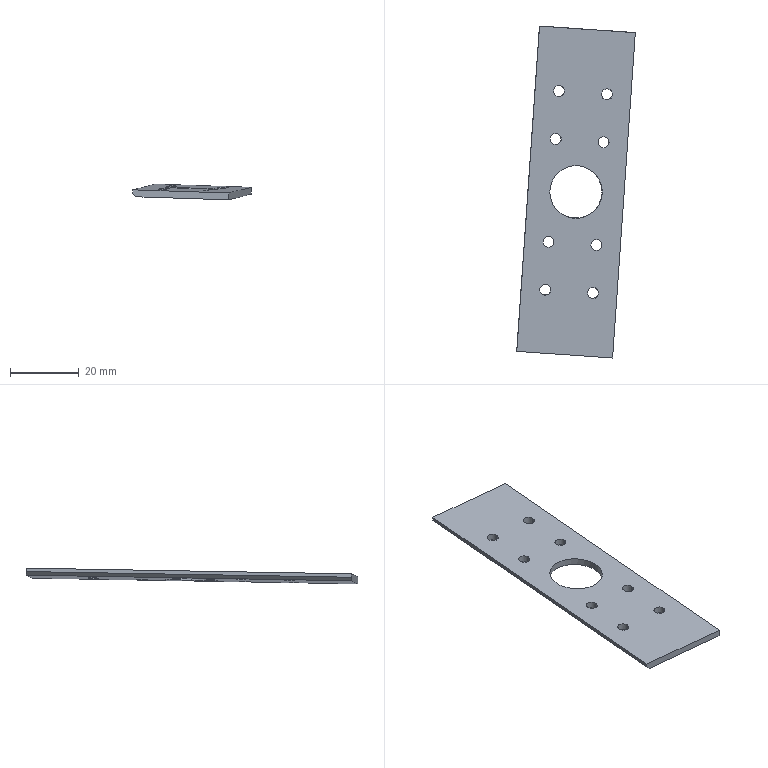Part | SolidWorks | features BaseBody 1 | 1 solid | 25 faces | box 34.576 x 96.71 x 4.578 mm | volume 4776 mm3 | cylinder 18 | plane 7 | commonest cylinder face diameters 3.2 x16 15.3 x2
STEP:
#1=CARTESIAN_POINT('',(-558.344,22.273,19.127));
#2=VERTEX_POINT('',#1);
#3=CARTESIAN_POINT('',(-561.543,22.273,19.228));
#4=VERTEX_POINT('',#3);
#5=CARTESIAN_POINT('',(-559.944,22.273,19.177));
#6=DIRECTION('',(-0.03175,0.01966,-0.9993));
#7=DIRECTION('',(0.9995,0.,-0.03176));
#8=AXIS2_PLACEMENT_3D('',#5,#6,#7);
#9=CIRCLE('',#8,1.6);
#10=EDGE_CURVE('',#2,#4,#9,.T.);
#11=ORIENTED_EDGE('',*,*,#10,.T.);
#12=CARTESIAN_POINT('',(-561.479,22.234,21.227));
#13=VERTEX_POINT('',#12);
#14=CARTESIAN_POINT('',(-561.543,22.273,19.228));
#15=DIRECTION('',(0.03175,-0.01966,0.9993));
#16=VECTOR('',#15,1000.);
#17=LINE('',#14,#16);
#18=EDGE_CURVE('',#4,#13,#17,.T.);
#19=ORIENTED_EDGE('',*,*,#18,.T.);
#20=CARTESIAN_POINT('',(-558.281,22.234,21.125));
#21=VERTEX_POINT('',#20);
#22=CARTESIAN_POINT('',(-559.88,22.234,21.176));
#23=DIRECTION('',(0.03175,-0.01966,0.9993));
#24=DIRECTION('',(0.9995,0.,-0.03176));
#25=AXIS2_PLACEMENT_3D('',#22,#23,#24);
#26=CIRCLE('',#25,1.6);
#27=EDGE_CURVE('',#13,#21,#26,.T.);
#28=ORIENTED_EDGE('',*,*,#27,.T.);
#29=CARTESIAN_POINT('',(-558.344,22.273,19.127));
#30=DIRECTION('',(0.03175,-0.01966,0.9993));
#31=VECTOR('',#30,1000.);
#32=LINE('',#29,#31);
#33=EDGE_CURVE('',#2,#21,#32,.T.);
#34=ORIENTED_EDGE('',*,*,#33,.F.);
#35=EDGE_LOOP('',(#11,#19,#28,#34));
#36=FACE_OUTER_BOUND('',#35,.T.);
#37=CARTESIAN_POINT('',(-559.944,22.273,19.177));
#38=DIRECTION('',(0.03175,-0.01966,0.9993));
#39=DIRECTION('',(0.9995,0.,-0.03176));
#40=AXIS2_PLACEMENT_3D('',#37,#38,#39);
#41=CYLINDRICAL_SURFACE('',#40,1.6);
#42=ADVANCED_FACE('',(#36),#41,.F.);
#43=CARTESIAN_POINT('',(-557.368,36.237,19.37));
#44=VERTEX_POINT('',#43);
#45=CARTESIAN_POINT('',(-560.566,36.237,19.472));
#46=VERTEX_POINT('',#45);
#47=CARTESIAN_POINT('',(-558.967,36.237,19.421));
#48=DIRECTION('',(-0.03175,0.01966,-0.9993));
#49=DIRECTION('',(0.9995,0.,-0.03176));
#50=AXIS2_PLACEMENT_3D('',#47,#48,#49);
#51=CIRCLE('',#50,1.6);
#52=EDGE_CURVE('',#44,#46,#51,.T.);
#53=ORIENTED_EDGE('',*,*,#52,.T.);
#54=CARTESIAN_POINT('',(-560.503,36.198,21.471));
#55=VERTEX_POINT('',#54);
#56=CARTESIAN_POINT('',(-560.566,36.237,19.472));
#57=DIRECTION('',(0.03175,-0.01966,0.9993));
#58=VECTOR('',#57,1000.);
#59=LINE('',#56,#58);
#60=EDGE_CURVE('',#46,#55,#59,.T.);
#61=ORIENTED_EDGE('',*,*,#60,.T.);
#62=CARTESIAN_POINT('',(-557.304,36.198,21.369));
#63=VERTEX_POINT('',#62);
#64=CARTESIAN_POINT('',(-558.903,36.198,21.42));
#65=DIRECTION('',(-0.03175,0.01966,-0.9993));
#66=DIRECTION('',(0.9995,0.,-0.03176));
#67=AXIS2_PLACEMENT_3D('',#64,#65,#66);
#68=CIRCLE('',#67,1.6);
#69=EDGE_CURVE('',#63,#55,#68,.T.);
#70=ORIENTED_EDGE('',*,*,#69,.F.);
#71=CARTESIAN_POINT('',(-557.368,36.237,19.37));
#72=DIRECTION('',(0.03175,-0.01966,0.9993));
#73=VECTOR('',#72,1000.);
#74=LINE('',#71,#73);
#75=EDGE_CURVE('',#44,#63,#74,.T.);
#76=ORIENTED_EDGE('',*,*,#75,.F.);
#77=EDGE_LOOP('',(#53,#61,#70,#76));
#78=FACE_OUTER_BOUND('',#77,.T.);
#79=CARTESIAN_POINT('',(-558.967,36.237,19.421));
#80=DIRECTION('',(0.03175,-0.01966,0.9993));
#81=DIRECTION('',(0.9995,0.,-0.03176));
#82=AXIS2_PLACEMENT_3D('',#79,#80,#81);
#83=CYLINDRICAL_SURFACE('',#82,1.6);
#84=ADVANCED_FACE('',(#78),#83,.F.);
#85=CARTESIAN_POINT('',(-554.299,80.119,20.136));
#86=VERTEX_POINT('',#85);
#87=CARTESIAN_POINT('',(-557.497,80.119,20.238));
#88=VERTEX_POINT('',#87);
#89=CARTESIAN_POINT('',(-555.898,80.119,20.187));
#90=DIRECTION('',(-0.03175,0.01966,-0.9993));
#91=DIRECTION('',(0.9995,0.,-0.03176));
#92=AXIS2_PLACEMENT_3D('',#89,#90,#91);
#93=CIRCLE('',#92,1.6);
#94=EDGE_CURVE('',#86,#88,#93,.T.);
#95=ORIENTED_EDGE('',*,*,#94,.T.);
#96=CARTESIAN_POINT('',(-557.434,80.079,22.237));
#97=VERTEX_POINT('',#96);
#98=CARTESIAN_POINT('',(-557.497,80.119,20.238));
#99=DIRECTION('',(0.03175,-0.01966,0.9993));
#100=VECTOR('',#99,1000.);
#101=LINE('',#98,#100);
#102=EDGE_CURVE('',#88,#97,#101,.T.);
#103=ORIENTED_EDGE('',*,*,#102,.T.);
#104=CARTESIAN_POINT('',(-554.235,80.079,22.135));
#105=VERTEX_POINT('',#104);
#106=CARTESIAN_POINT('',(-555.834,80.079,22.186));
#107=DIRECTION('',(-0.03175,0.01966,-0.9993));
#108=DIRECTION('',(0.9995,0.,-0.03176));
#109=AXIS2_PLACEMENT_3D('',#106,#107,#108);
#110=CIRCLE('',#109,1.6);
#111=EDGE_CURVE('',#105,#97,#110,.T.);
#112=ORIENTED_EDGE('',*,*,#111,.F.);
#113=CARTESIAN_POINT('',(-554.299,80.119,20.136));
#114=DIRECTION('',(0.03175,-0.01966,0.9993));
#115=VECTOR('',#114,1000.);
#116=LINE('',#113,#115);
#117=EDGE_CURVE('',#86,#105,#116,.T.);
#118=ORIENTED_EDGE('',*,*,#117,.F.);
#119=EDGE_LOOP('',(#95,#103,#112,#118));
#120=FACE_OUTER_BOUND('',#119,.T.);
#121=CARTESIAN_POINT('',(-555.898,80.119,20.187));
#122=DIRECTION('',(0.03175,-0.01966,0.9993));
#123=DIRECTION('',(0.9995,0.,-0.03176));
#124=AXIS2_PLACEMENT_3D('',#121,#122,#123);
#125=CYLINDRICAL_SURFACE('',#124,1.6);
#126=ADVANCED_FACE('',(#120),#125,.F.);
#127=CARTESIAN_POINT('',(-569.234,67.123,20.355));
#128=VERTEX_POINT('',#127);
#129=CARTESIAN_POINT('',(-572.433,67.123,20.457));
#130=VERTEX_POINT('',#129);
#131=CARTESIAN_POINT('',(-570.833,67.123,20.406));
#132=DIRECTION('',(-0.03175,0.01966,-0.9993));
#133=DIRECTION('',(0.9995,0.,-0.03176));
#134=AXIS2_PLACEMENT_3D('',#131,#132,#133);
#135=CIRCLE('',#134,1.6);
#136=EDGE_CURVE('',#128,#130,#135,.T.);
#137=ORIENTED_EDGE('',*,*,#136,.T.);
#138=CARTESIAN_POINT('',(-572.369,67.084,22.455));
#139=VERTEX_POINT('',#138);
#140=CARTESIAN_POINT('',(-572.433,67.123,20.457));
#141=DIRECTION('',(0.03175,-0.01966,0.9993));
#142=VECTOR('',#141,1000.);
#143=LINE('',#140,#142);
#144=EDGE_CURVE('',#130,#139,#143,.T.);
#145=ORIENTED_EDGE('',*,*,#144,.T.);
#146=CARTESIAN_POINT('',(-569.171,67.084,22.354));
#147=VERTEX_POINT('',#146);
#148=CARTESIAN_POINT('',(-570.77,67.084,22.405));
#149=DIRECTION('',(-0.03175,0.01966,-0.9993));
#150=DIRECTION('',(0.9995,0.,-0.03176));
#151=AXIS2_PLACEMENT_3D('',#148,#149,#150);
#152=CIRCLE('',#151,1.6);
#153=EDGE_CURVE('',#147,#139,#152,.T.);
#154=ORIENTED_EDGE('',*,*,#153,.F.);
#155=CARTESIAN_POINT('',(-569.234,67.123,20.355));
#156=DIRECTION('',(0.03175,-0.01966,0.9993));
#157=VECTOR('',#156,1000.);
#158=LINE('',#155,#157);
#159=EDGE_CURVE('',#128,#147,#158,.T.);
#160=ORIENTED_EDGE('',*,*,#159,.F.);
#161=EDGE_LOOP('',(#137,#145,#154,#160));
#162=FACE_OUTER_BOUND('',#161,.T.);
#163=CARTESIAN_POINT('',(-570.833,67.123,20.406));
#164=DIRECTION('',(0.03175,-0.01966,0.9993));
#165=DIRECTION('',(0.9995,0.,-0.03176));
#166=AXIS2_PLACEMENT_3D('',#163,#164,#165);
#167=CYLINDRICAL_SURFACE('',#166,1.6);
#168=ADVANCED_FACE('',(#162),#167,.F.);
#169=CARTESIAN_POINT('',(-557.254,51.68,19.671));
#170=VERTEX_POINT('',#169);
#171=CARTESIAN_POINT('',(-572.546,51.68,20.157));
#172=VERTEX_POINT('',#171);
#173=CARTESIAN_POINT('',(-564.9,51.68,19.914));
#174=DIRECTION('',(-0.03175,0.01966,-0.9993));
#175=DIRECTION('',(0.9995,0.,-0.03176));
#176=AXIS2_PLACEMENT_3D('',#173,#174,#175);
#177=CIRCLE('',#176,7.65);
#178=EDGE_CURVE('',#170,#172,#177,.T.);
#179=ORIENTED_EDGE('',*,*,#178,.T.);
#180=CARTESIAN_POINT('',(-572.483,51.641,22.155));
#181=VERTEX_POINT('',#180);
#182=CARTESIAN_POINT('',(-572.546,51.68,20.157));
#183=DIRECTION('',(0.03175,-0.01966,0.9993));
#184=VECTOR('',#183,1000.);
#185=LINE('',#182,#184);
#186=EDGE_CURVE('',#172,#181,#185,.T.);
#187=ORIENTED_EDGE('',*,*,#186,.T.);
#188=CARTESIAN_POINT('',(-557.191,51.641,21.669));
#189=VERTEX_POINT('',#188);
#190=CARTESIAN_POINT('',(-564.837,51.641,21.912));
#191=DIRECTION('',(-0.03175,0.01966,-0.9993));
#192=DIRECTION('',(0.9995,0.,-0.03176));
#193=AXIS2_PLACEMENT_3D('',#190,#191,#192);
#194=CIRCLE('',#193,7.65);
#195=EDGE_CURVE('',#189,#181,#194,.T.);
#196=ORIENTED_EDGE('',*,*,#195,.F.);
#197=CARTESIAN_POINT('',(-557.254,51.68,19.671));
#198=DIRECTION('',(0.03175,-0.01966,0.9993));
#199=VECTOR('',#198,1000.);
#200=LINE('',#197,#199);
#201=EDGE_CURVE('',#170,#189,#200,.T.);
#202=ORIENTED_EDGE('',*,*,#201,.F.);
#203=EDGE_LOOP('',(#179,#187,#196,#202));
#204=FACE_OUTER_BOUND('',#203,.T.);
#205=CARTESIAN_POINT('',(-564.9,51.68,19.914));
#206=DIRECTION('',(0.03175,-0.01966,0.9993));
#207=DIRECTION('',(0.9995,0.,-0.03176));
#208=AXIS2_PLACEMENT_3D('',#205,#206,#207);
#209=CYLINDRICAL_SURFACE('',#208,7.65);
#210=ADVANCED_FACE('',(#204),#209,.F.);
#211=CARTESIAN_POINT('',(-555.275,66.155,19.893));
#212=VERTEX_POINT('',#211);
#213=CARTESIAN_POINT('',(-558.474,66.155,19.994));
#214=VERTEX_POINT('',#213);
#215=CARTESIAN_POINT('',(-556.875,66.155,19.943));
#216=DIRECTION('',(-0.03175,0.01966,-0.9993));
#217=DIRECTION('',(0.9995,0.,-0.03176));
#218=AXIS2_PLACEMENT_3D('',#215,#216,#217);
#219=CIRCLE('',#218,1.6);
#220=EDGE_CURVE('',#212,#214,#219,.T.);
#221=ORIENTED_EDGE('',*,*,#220,.T.);
#222=CARTESIAN_POINT('',(-558.41,66.116,21.993));
#223=VERTEX_POINT('',#222);
#224=CARTESIAN_POINT('',(-558.474,66.155,19.994));
#225=DIRECTION('',(0.03175,-0.01966,0.9993));
#226=VECTOR('',#225,1000.);
#227=LINE('',#224,#226);
#228=EDGE_CURVE('',#214,#223,#227,.T.);
#229=ORIENTED_EDGE('',*,*,#228,.T.);
#230=CARTESIAN_POINT('',(-555.212,66.116,21.891));
#231=VERTEX_POINT('',#230);
#232=CARTESIAN_POINT('',(-556.811,66.116,21.942));
#233=DIRECTION('',(-0.03175,0.01966,-0.9993));
#234=DIRECTION('',(0.9995,0.,-0.03176));
#235=AXIS2_PLACEMENT_3D('',#232,#233,#234);
#236=CIRCLE('',#235,1.6);
#237=EDGE_CURVE('',#231,#223,#236,.T.);
#238=ORIENTED_EDGE('',*,*,#237,.F.);
#239=CARTESIAN_POINT('',(-555.275,66.155,19.893));
#240=DIRECTION('',(0.03175,-0.01966,0.9993));
#241=VECTOR('',#240,1000.);
#242=LINE('',#239,#241);
#243=EDGE_CURVE('',#212,#231,#242,.T.);
#244=ORIENTED_EDGE('',*,*,#243,.F.);
#245=EDGE_LOOP('',(#221,#229,#238,#244));
#246=FACE_OUTER_BOUND('',#245,.T.);
#247=CARTESIAN_POINT('',(-556.875,66.155,19.943));
#248=DIRECTION('',(0.03175,-0.01966,0.9993));
#249=DIRECTION('',(0.9995,0.,-0.03176));
#250=AXIS2_PLACEMENT_3D('',#247,#248,#249);
#251=CYLINDRICAL_SURFACE('',#250,1.6);
#252=ADVANCED_FACE('',(#246),#251,.F.);
#253=CARTESIAN_POINT('',(-568.258,81.087,20.599));
#254=VERTEX_POINT('',#253);
#255=CARTESIAN_POINT('',(-571.456,81.087,20.701));
#256=VERTEX_POINT('',#255);
#257=CARTESIAN_POINT('',(-569.857,81.087,20.65));
#258=DIRECTION('',(-0.03175,0.01966,-0.9993));
#259=DIRECTION('',(0.9995,0.,-0.03176));
#260=AXIS2_PLACEMENT_3D('',#257,#258,#259);
#261=CIRCLE('',#260,1.6);
#262=EDGE_CURVE('',#254,#256,#261,.T.);
#263=ORIENTED_EDGE('',*,*,#262,.T.);
#264=CARTESIAN_POINT('',(-571.393,81.048,22.699));
#265=VERTEX_POINT('',#264);
#266=CARTESIAN_POINT('',(-571.456,81.087,20.701));
#267=DIRECTION('',(0.03175,-0.01966,0.9993));
#268=VECTOR('',#267,1000.);
#269=LINE('',#266,#268);
#270=EDGE_CURVE('',#256,#265,#269,.T.);
#271=ORIENTED_EDGE('',*,*,#270,.T.);
#272=CARTESIAN_POINT('',(-568.194,81.048,22.598));
#273=VERTEX_POINT('',#272);
#274=CARTESIAN_POINT('',(-569.793,81.048,22.648));
#275=DIRECTION('',(-0.03175,0.01966,-0.9993));
#276=DIRECTION('',(0.9995,0.,-0.03176));
#277=AXIS2_PLACEMENT_3D('',#274,#275,#276);
#278=CIRCLE('',#277,1.6);
#279=EDGE_CURVE('',#273,#265,#278,.T.);
#280=ORIENTED_EDGE('',*,*,#279,.F.);
#281=CARTESIAN_POINT('',(-568.258,81.087,20.599));
#282=DIRECTION('',(0.03175,-0.01966,0.9993));
#283=VECTOR('',#282,1000.);
#284=LINE('',#281,#283);
#285=EDGE_CURVE('',#254,#273,#284,.T.);
#286=ORIENTED_EDGE('',*,*,#285,.F.);
#287=EDGE_LOOP('',(#263,#271,#280,#286));
#288=FACE_OUTER_BOUND('',#287,.T.);
#289=CARTESIAN_POINT('',(-569.857,81.087,20.65));
#290=DIRECTION('',(0.03175,-0.01966,0.9993));
#291=DIRECTION('',(0.9995,0.,-0.03176));
#292=AXIS2_PLACEMENT_3D('',#289,#290,#291);
#293=CYLINDRICAL_SURFACE('',#292,1.6);
#294=ADVANCED_FACE('',(#288),#293,.F.);
#295=CARTESIAN_POINT('',(-571.327,37.205,19.833));
#296=VERTEX_POINT('',#295);
#297=CARTESIAN_POINT('',(-574.525,37.205,19.935));
#298=VERTEX_POINT('',#297);
#299=CARTESIAN_POINT('',(-572.926,37.205,19.884));
#300=DIRECTION('',(-0.03175,0.01966,-0.9993));
#301=DIRECTION('',(0.9995,0.,-0.03176));
#302=AXIS2_PLACEMENT_3D('',#299,#300,#301);
#303=CIRCLE('',#302,1.6);
#304=EDGE_CURVE('',#296,#298,#303,.T.);
#305=ORIENTED_EDGE('',*,*,#304,.T.);
#306=CARTESIAN_POINT('',(-574.461,37.166,21.933));
#307=VERTEX_POINT('',#306);
#308=CARTESIAN_POINT('',(-574.525,37.205,19.935));
#309=DIRECTION('',(0.03175,-0.01966,0.9993));
#310=VECTOR('',#309,1000.);
#311=LINE('',#308,#310);
#312=EDGE_CURVE('',#298,#307,#311,.T.);
#313=ORIENTED_EDGE('',*,*,#312,.T.);
#314=CARTESIAN_POINT('',(-571.263,37.166,21.832));
#315=VERTEX_POINT('',#314);
#316=CARTESIAN_POINT('',(-572.862,37.166,21.882));
#317=DIRECTION('',(-0.03175,0.01966,-0.9993));
#318=DIRECTION('',(0.9995,0.,-0.03176));
#319=AXIS2_PLACEMENT_3D('',#316,#317,#318);
#320=CIRCLE('',#319,1.6);
#321=EDGE_CURVE('',#315,#307,#320,.T.);
#322=ORIENTED_EDGE('',*,*,#321,.F.);
#323=CARTESIAN_POINT('',(-571.327,37.205,19.833));
#324=DIRECTION('',(0.03175,-0.01966,0.9993));
#325=VECTOR('',#324,1000.);
#326=LINE('',#323,#325);
#327=EDGE_CURVE('',#296,#315,#326,.T.);
#328=ORIENTED_EDGE('',*,*,#327,.F.);
#329=EDGE_LOOP('',(#305,#313,#322,#328));
#330=FACE_OUTER_BOUND('',#329,.T.);
#331=CARTESIAN_POINT('',(-572.926,37.205,19.884));
#332=DIRECTION('',(0.03175,-0.01966,0.9993));
#333=DIRECTION('',(0.9995,0.,-0.03176));
#334=AXIS2_PLACEMENT_3D('',#331,#332,#333);
#335=CYLINDRICAL_SURFACE('',#334,1.6);
#336=ADVANCED_FACE('',(#330),#335,.F.);
#337=CARTESIAN_POINT('',(-572.303,23.242,19.589));
#338=VERTEX_POINT('',#337);
#339=CARTESIAN_POINT('',(-575.502,23.242,19.691));
#340=VERTEX_POINT('',#339);
#341=CARTESIAN_POINT('',(-573.902,23.242,19.64));
#342=DIRECTION('',(-0.03175,0.01966,-0.9993));
#343=DIRECTION('',(0.9995,0.,-0.03176));
#344=AXIS2_PLACEMENT_3D('',#341,#342,#343);
#345=CIRCLE('',#344,1.6);
#346=EDGE_CURVE('',#338,#340,#345,.T.);
#347=ORIENTED_EDGE('',*,*,#346,.T.);
#348=CARTESIAN_POINT('',(-575.438,23.202,21.689));
#349=VERTEX_POINT('',#348);
#350=CARTESIAN_POINT('',(-575.502,23.242,19.691));
#351=DIRECTION('',(0.03175,-0.01966,0.9993));
#352=VECTOR('',#351,1000.);
#353=LINE('',#350,#352);
#354=EDGE_CURVE('',#340,#349,#353,.T.);
#355=ORIENTED_EDGE('',*,*,#354,.T.);
#356=CARTESIAN_POINT('',(-572.24,23.202,21.588));
#357=VERTEX_POINT('',#356);
#358=CARTESIAN_POINT('',(-573.839,23.202,21.639));
#359=DIRECTION('',(-0.03175,0.01966,-0.9993));
#360=DIRECTION('',(0.9995,0.,-0.03176));
#361=AXIS2_PLACEMENT_3D('',#358,#359,#360);
#362=CIRCLE('',#361,1.6);
#363=EDGE_CURVE('',#357,#349,#362,.T.);
#364=ORIENTED_EDGE('',*,*,#363,.F.);
#365=CARTESIAN_POINT('',(-572.303,23.242,19.589));
#366=DIRECTION('',(0.03175,-0.01966,0.9993));
#367=VECTOR('',#366,1000.);
#368=LINE('',#365,#367);
#369=EDGE_CURVE('',#338,#357,#368,.T.);
#370=ORIENTED_EDGE('',*,*,#369,.F.);
#371=EDGE_LOOP('',(#347,#355,#364,#370));
#372=FACE_OUTER_BOUND('',#371,.T.);
#373=CARTESIAN_POINT('',(-573.902,23.242,19.64));
#374=DIRECTION('',(0.03175,-0.01966,0.9993));
#375=DIRECTION('',(0.9995,0.,-0.03176));
#376=AXIS2_PLACEMENT_3D('',#373,#374,#375);
#377=CYLINDRICAL_SURFACE('',#376,1.6);
#378=ADVANCED_FACE('',(#372),#377,.F.);
#379=ORIENTED_EDGE('',*,*,#18,.F.);
#380=CARTESIAN_POINT('',(-559.944,22.273,19.177));
#381=DIRECTION('',(-0.03175,0.01966,-0.9993));
#382=DIRECTION('',(0.9995,0.,-0.03176));
#383=AXIS2_PLACEMENT_3D('',#380,#381,#382);
#384=CIRCLE('',#383,1.6);
#385=EDGE_CURVE('',#4,#2,#384,.T.);
#386=ORIENTED_EDGE('',*,*,#385,.T.);
#387=ORIENTED_EDGE('',*,*,#33,.T.);
#388=CARTESIAN_POINT('',(-559.88,22.234,21.176));
#389=DIRECTION('',(0.03175,-0.01966,0.9993));
#390=DIRECTION('',(0.9995,0.,-0.03176));
#391=AXIS2_PLACEMENT_3D('',#388,#389,#390);
#392=CIRCLE('',#391,1.6);
#393=EDGE_CURVE('',#21,#13,#392,.T.);
#394=ORIENTED_EDGE('',*,*,#393,.T.);
#395=EDGE_LOOP('',(#379,#386,#387,#394));
#396=FACE_OUTER_BOUND('',#395,.T.);
#397=CARTESIAN_POINT('',(-559.944,22.273,19.177));
#398=DIRECTION('',(0.03175,-0.01966,0.9993));
#399=DIRECTION('',(0.9995,0.,-0.03176));
#400=AXIS2_PLACEMENT_3D('',#397,#398,#399);
#401=CYLINDRICAL_SURFACE('',#400,1.6);
#402=ADVANCED_FACE('',(#396),#401,.F.);
#403=ORIENTED_EDGE('',*,*,#393,.F.);
#404=ORIENTED_EDGE('',*,*,#27,.F.);
#405=EDGE_LOOP('',(#403,#404));
#406=FACE_BOUND('',#405,.T.);
#407=ORIENTED_EDGE('',*,*,#69,.T.);
#408=CARTESIAN_POINT('',(-558.903,36.198,21.42));
#409=DIRECTION('',(-0.03175,0.01966,-0.9993));
#410=DIRECTION('',(0.9995,0.,-0.03176));
#411=AXIS2_PLACEMENT_3D('',#408,#409,#410);
#412=CIRCLE('',#411,1.6);
#413=EDGE_CURVE('',#55,#63,#412,.T.);
#414=ORIENTED_EDGE('',*,*,#413,.T.);
#415=EDGE_LOOP('',(#407,#414));
#416=FACE_BOUND('',#415,.T.);
#417=ORIENTED_EDGE('',*,*,#111,.T.);
#418=CARTESIAN_POINT('',(-555.834,80.079,22.186));
#419=DIRECTION('',(-0.03175,0.01966,-0.9993));
#420=DIRECTION('',(0.9995,0.,-0.03176));
#421=AXIS2_PLACEMENT_3D('',#418,#419,#420);
#422=CIRCLE('',#421,1.6);
#423=EDGE_CURVE('',#97,#105,#422,.T.);
#424=ORIENTED_EDGE('',*,*,#423,.T.);
#425=EDGE_LOOP('',(#417,#424));
#426=FACE_BOUND('',#425,.T.);
#427=ORIENTED_EDGE('',*,*,#153,.T.);
#428=CARTESIAN_POINT('',(-570.77,67.084,22.405));
#429=DIRECTION('',(-0.03175,0.01966,-0.9993));
#430=DIRECTION('',(0.9995,0.,-0.03176));
#431=AXIS2_PLACEMENT_3D('',#428,#429,#430);
#432=CIRCLE('',#431,1.6);
#433=EDGE_CURVE('',#139,#147,#432,.T.);
#434=ORIENTED_EDGE('',*,*,#433,.T.);
#435=EDGE_LOOP('',(#427,#434));
#436=FACE_BOUND('',#435,.T.);
#437=ORIENTED_EDGE('',*,*,#195,.T.);
#438=CARTESIAN_POINT('',(-564.837,51.641,21.912));
#439=DIRECTION('',(-0.03175,0.01966,-0.9993));
#440=DIRECTION('',(0.9995,0.,-0.03176));
#441=AXIS2_PLACEMENT_3D('',#438,#439,#440);
#442=CIRCLE('',#441,7.65);
#443=EDGE_CURVE('',#181,#189,#442,.T.);
#444=ORIENTED_EDGE('',*,*,#443,.T.);
#445=EDGE_LOOP('',(#437,#444));
#446=FACE_BOUND('',#445,.T.);
#447=ORIENTED_EDGE('',*,*,#237,.T.);
#448=CARTESIAN_POINT('',(-556.811,66.116,21.942));
#449=DIRECTION('',(-0.03175,0.01966,-0.9993));
#450=DIRECTION('',(0.9995,0.,-0.03176));
#451=AXIS2_PLACEMENT_3D('',#448,#449,#450);
#452=CIRCLE('',#451,1.6);
#453=EDGE_CURVE('',#223,#231,#452,.T.);
#454=ORIENTED_EDGE('',*,*,#453,.T.);
#455=EDGE_LOOP('',(#447,#454));
#456=FACE_BOUND('',#455,.T.);
#457=ORIENTED_EDGE('',*,*,#279,.T.);
#458=CARTESIAN_POINT('',(-569.793,81.048,22.648));
#459=DIRECTION('',(-0.03175,0.01966,-0.9993));
#460=DIRECTION('',(0.9995,0.,-0.03176));
#461=AXIS2_PLACEMENT_3D('',#458,#459,#460);
#462=CIRCLE('',#461,1.6);
#463=EDGE_CURVE('',#265,#273,#462,.T.);
#464=ORIENTED_EDGE('',*,*,#463,.T.);
#465=EDGE_LOOP('',(#457,#464));
#466=FACE_BOUND('',#465,.T.);
#467=ORIENTED_EDGE('',*,*,#321,.T.);
#468=CARTESIAN_POINT('',(-572.862,37.166,21.882));
#469=DIRECTION('',(-0.03175,0.01966,-0.9993));
#470=DIRECTION('',(0.9995,0.,-0.03176));
#471=AXIS2_PLACEMENT_3D('',#468,#469,#470);
#472=CIRCLE('',#471,1.6);
#473=EDGE_CURVE('',#307,#315,#472,.T.);
#474=ORIENTED_EDGE('',*,*,#473,.T.);
#475=EDGE_LOOP('',(#467,#474));
#476=FACE_BOUND('',#475,.T.);
#477=ORIENTED_EDGE('',*,*,#363,.T.);
#478=CARTESIAN_POINT('',(-573.839,23.202,21.639));
#479=DIRECTION('',(-0.03175,0.01966,-0.9993));
#480=DIRECTION('',(0.9995,0.,-0.03176));
#481=AXIS2_PLACEMENT_3D('',#478,#479,#480);
#482=CIRCLE('',#481,1.6);
#483=EDGE_CURVE('',#349,#357,#482,.T.);
#484=ORIENTED_EDGE('',*,*,#483,.T.);
#485=EDGE_LOOP('',(#477,#484));
#486=FACE_BOUND('',#485,.T.);
#487=CARTESIAN_POINT('',(-582.109,5.232,21.548));
#488=VERTEX_POINT('',#487);
#489=CARTESIAN_POINT('',(-554.191,3.296,20.623));
#490=VERTEX_POINT('',#489);
#491=CARTESIAN_POINT('',(-582.109,5.232,21.548));
#492=DIRECTION('',(0.9971,-0.06916,-0.03304));
#493=VECTOR('',#492,1000.);
#494=LINE('',#491,#493);
#495=EDGE_CURVE('',#488,#490,#494,.T.);
#496=ORIENTED_EDGE('',*,*,#495,.T.);
#497=CARTESIAN_POINT('',(-547.564,98.05,22.277));
#498=VERTEX_POINT('',#497);
#499=CARTESIAN_POINT('',(-554.191,3.296,20.623));
#500=DIRECTION('',(0.06976,0.9974,0.01741));
#501=VECTOR('',#500,1000.);
#502=LINE('',#499,#501);
#503=EDGE_CURVE('',#490,#498,#502,.T.);
#504=ORIENTED_EDGE('',*,*,#503,.T.);
#505=CARTESIAN_POINT('',(-575.482,99.986,23.202));
#506=VERTEX_POINT('',#505);
#507=CARTESIAN_POINT('',(-547.564,98.05,22.277));
#508=DIRECTION('',(-0.9971,0.06916,0.03304));
#509=VECTOR('',#508,1000.);
#510=LINE('',#507,#509);
#511=EDGE_CURVE('',#498,#506,#510,.T.);
#512=ORIENTED_EDGE('',*,*,#511,.T.);
#513=CARTESIAN_POINT('',(-575.482,99.986,23.202));
#514=DIRECTION('',(-0.06976,-0.9974,-0.01741));
#515=VECTOR('',#514,1000.);
#516=LINE('',#513,#515);
#517=EDGE_CURVE('',#506,#488,#516,.T.);
#518=ORIENTED_EDGE('',*,*,#517,.T.);
#519=EDGE_LOOP('',(#496,#504,#512,#518));
#520=FACE_OUTER_BOUND('',#519,.T.);
#521=CARTESIAN_POINT('',(-582.317,2.715,21.505));
#522=DIRECTION('',(0.03175,-0.01966,0.9993));
#523=DIRECTION('',(0.9995,0.,-0.03176));
#524=AXIS2_PLACEMENT_3D('',#521,#522,#523);
#525=PLANE('',#524);
#526=ADVANCED_FACE('',(#406,#416,#426,#436,#446,#456,#466,#476,#486,#520),#525,.T.);
#527=ORIENTED_EDGE('',*,*,#10,.F.);
#528=ORIENTED_EDGE('',*,*,#385,.F.);
#529=EDGE_LOOP('',(#527,#528));
#530=FACE_BOUND('',#529,.T.);
#531=ORIENTED_EDGE('',*,*,#52,.F.);
#532=CARTESIAN_POINT('',(-558.967,36.237,19.421));
#533=DIRECTION('',(-0.03175,0.01966,-0.9993));
#534=DIRECTION('',(0.9995,0.,-0.03176));
#535=AXIS2_PLACEMENT_3D('',#532,#533,#534);
#536=CIRCLE('',#535,1.6);
#537=EDGE_CURVE('',#46,#44,#536,.T.);
#538=ORIENTED_EDGE('',*,*,#537,.F.);
#539=EDGE_LOOP('',(#531,#538));
#540=FACE_BOUND('',#539,.T.);
#541=ORIENTED_EDGE('',*,*,#94,.F.);
#542=CARTESIAN_POINT('',(-555.898,80.119,20.187));
#543=DIRECTION('',(-0.03175,0.01966,-0.9993));
#544=DIRECTION('',(0.9995,0.,-0.03176));
#545=AXIS2_PLACEMENT_3D('',#542,#543,#544);
#546=CIRCLE('',#545,1.6);
#547=EDGE_CURVE('',#88,#86,#546,.T.);
#548=ORIENTED_EDGE('',*,*,#547,.F.);
#549=EDGE_LOOP('',(#541,#548));
#550=FACE_BOUND('',#549,.T.);
#551=ORIENTED_EDGE('',*,*,#136,.F.);
#552=CARTESIAN_POINT('',(-570.833,67.123,20.406));
#553=DIRECTION('',(-0.03175,0.01966,-0.9993));
#554=DIRECTION('',(0.9995,0.,-0.03176));
#555=AXIS2_PLACEMENT_3D('',#552,#553,#554);
#556=CIRCLE('',#555,1.6);
#557=EDGE_CURVE('',#130,#128,#556,.T.);
#558=ORIENTED_EDGE('',*,*,#557,.F.);
#559=EDGE_LOOP('',(#551,#558));
#560=FACE_BOUND('',#559,.T.);
#561=ORIENTED_EDGE('',*,*,#178,.F.);
#562=CARTESIAN_POINT('',(-564.9,51.68,19.914));
#563=DIRECTION('',(-0.03175,0.01966,-0.9993));
#564=DIRECTION('',(0.9995,0.,-0.03176));
#565=AXIS2_PLACEMENT_3D('',#562,#563,#564);
#566=CIRCLE('',#565,7.65);
#567=EDGE_CURVE('',#172,#170,#566,.T.);
#568=ORIENTED_EDGE('',*,*,#567,.F.);
#569=EDGE_LOOP('',(#561,#568));
#570=FACE_BOUND('',#569,.T.);
#571=ORIENTED_EDGE('',*,*,#220,.F.);
#572=CARTESIAN_POINT('',(-556.875,66.155,19.943));
#573=DIRECTION('',(-0.03175,0.01966,-0.9993));
#574=DIRECTION('',(0.9995,0.,-0.03176));
#575=AXIS2_PLACEMENT_3D('',#572,#573,#574);
#576=CIRCLE('',#575,1.6);
#577=EDGE_CURVE('',#214,#212,#576,.T.);
#578=ORIENTED_EDGE('',*,*,#577,.F.);
#579=EDGE_LOOP('',(#571,#578));
#580=FACE_BOUND('',#579,.T.);
#581=ORIENTED_EDGE('',*,*,#262,.F.);
#582=CARTESIAN_POINT('',(-569.857,81.087,20.65));
#583=DIRECTION('',(-0.03175,0.01966,-0.9993));
#584=DIRECTION('',(0.9995,0.,-0.03176));
#585=AXIS2_PLACEMENT_3D('',#582,#583,#584);
#586=CIRCLE('',#585,1.6);
#587=EDGE_CURVE('',#256,#254,#586,.T.);
#588=ORIENTED_EDGE('',*,*,#587,.F.);
#589=EDGE_LOOP('',(#581,#588));
#590=FACE_BOUND('',#589,.T.);
#591=ORIENTED_EDGE('',*,*,#304,.F.);
#592=CARTESIAN_POINT('',(-572.926,37.205,19.884));
#593=DIRECTION('',(-0.03175,0.01966,-0.9993));
#594=DIRECTION('',(0.9995,0.,-0.03176));
#595=AXIS2_PLACEMENT_3D('',#592,#593,#594);
#596=CIRCLE('',#595,1.6);
#597=EDGE_CURVE('',#298,#296,#596,.T.);
#598=ORIENTED_EDGE('',*,*,#597,.F.);
#599=EDGE_LOOP('',(#591,#598));
#600=FACE_BOUND('',#599,.T.);
#601=ORIENTED_EDGE('',*,*,#346,.F.);
#602=CARTESIAN_POINT('',(-573.902,23.242,19.64));
#603=DIRECTION('',(-0.03175,0.01966,-0.9993));
#604=DIRECTION('',(0.9995,0.,-0.03176));
#605=AXIS2_PLACEMENT_3D('',#602,#603,#604);
#606=CIRCLE('',#605,1.6);
#607=EDGE_CURVE('',#340,#338,#606,.T.);
#608=ORIENTED_EDGE('',*,*,#607,.F.);
#609=EDGE_LOOP('',(#601,#608));
#610=FACE_BOUND('',#609,.T.);
#611=CARTESIAN_POINT('',(-574.549,99.956,21.17));
#612=VERTEX_POINT('',#611);
#613=CARTESIAN_POINT('',(-581.175,5.202,19.516));
#614=VERTEX_POINT('',#613);
#615=CARTESIAN_POINT('',(-574.549,99.956,21.17));
#616=DIRECTION('',(-0.06976,-0.9974,-0.01741));
#617=VECTOR('',#616,1000.);
#618=LINE('',#615,#617);
#619=EDGE_CURVE('',#612,#614,#618,.T.);
#620=ORIENTED_EDGE('',*,*,#619,.F.);
#621=CARTESIAN_POINT('',(-547.628,98.089,20.278));
#622=VERTEX_POINT('',#621);
#623=CARTESIAN_POINT('',(-547.628,98.089,20.278));
#624=DIRECTION('',(-0.9971,0.06916,0.03304));
#625=VECTOR('',#624,1000.);
#626=LINE('',#623,#625);
#627=EDGE_CURVE('',#622,#612,#626,.T.);
#628=ORIENTED_EDGE('',*,*,#627,.F.);
#629=CARTESIAN_POINT('',(-554.255,3.335,18.624));
#630=VERTEX_POINT('',#629);
#631=CARTESIAN_POINT('',(-554.255,3.335,18.624));
#632=DIRECTION('',(0.06976,0.9974,0.01741));
#633=VECTOR('',#632,1000.);
#634=LINE('',#631,#633);
#635=EDGE_CURVE('',#630,#622,#634,.T.);
#636=ORIENTED_EDGE('',*,*,#635,.F.);
#637=CARTESIAN_POINT('',(-581.175,5.202,19.516));
#638=DIRECTION('',(0.9971,-0.06916,-0.03304));
#639=VECTOR('',#638,1000.);
#640=LINE('',#637,#639);
#641=EDGE_CURVE('',#614,#630,#640,.T.);
#642=ORIENTED_EDGE('',*,*,#641,.F.);
#643=EDGE_LOOP('',(#620,#628,#636,#642));
#644=FACE_OUTER_BOUND('',#643,.T.);
#645=CARTESIAN_POINT('',(-581.378,2.755,19.474));
#646=DIRECTION('',(0.03175,-0.01966,0.9993));
#647=DIRECTION('',(0.9995,0.,-0.03176));
#648=AXIS2_PLACEMENT_3D('',#645,#646,#647);
#649=PLANE('',#648);
#650=ADVANCED_FACE('',(#530,#540,#550,#560,#570,#580,#590,#600,#610,#644),#649,.F.);
#651=ORIENTED_EDGE('',*,*,#60,.F.);
#652=ORIENTED_EDGE('',*,*,#537,.T.);
#653=ORIENTED_EDGE('',*,*,#75,.T.);
#654=ORIENTED_EDGE('',*,*,#413,.F.);
#655=EDGE_LOOP('',(#651,#652,#653,#654));
#656=FACE_OUTER_BOUND('',#655,.T.);
#657=CARTESIAN_POINT('',(-558.967,36.237,19.421));
#658=DIRECTION('',(0.03175,-0.01966,0.9993));
#659=DIRECTION('',(0.9995,0.,-0.03176));
#660=AXIS2_PLACEMENT_3D('',#657,#658,#659);
#661=CYLINDRICAL_SURFACE('',#660,1.6);
#662=ADVANCED_FACE('',(#656),#661,.F.);
#663=ORIENTED_EDGE('',*,*,#102,.F.);
#664=ORIENTED_EDGE('',*,*,#547,.T.);
#665=ORIENTED_EDGE('',*,*,#117,.T.);
#666=ORIENTED_EDGE('',*,*,#423,.F.);
#667=EDGE_LOOP('',(#663,#664,#665,#666));
#668=FACE_OUTER_BOUND('',#667,.T.);
#669=CARTESIAN_POINT('',(-555.898,80.119,20.187));
#670=DIRECTION('',(0.03175,-0.01966,0.9993));
#671=DIRECTION('',(0.9995,0.,-0.03176));
#672=AXIS2_PLACEMENT_3D('',#669,#670,#671);
#673=CYLINDRICAL_SURFACE('',#672,1.6);
#674=ADVANCED_FACE('',(#668),#673,.F.);
#675=ORIENTED_EDGE('',*,*,#144,.F.);
#676=ORIENTED_EDGE('',*,*,#557,.T.);
#677=ORIENTED_EDGE('',*,*,#159,.T.);
#678=ORIENTED_EDGE('',*,*,#433,.F.);
#679=EDGE_LOOP('',(#675,#676,#677,#678));
#680=FACE_OUTER_BOUND('',#679,.T.);
#681=CARTESIAN_POINT('',(-570.833,67.123,20.406));
#682=DIRECTION('',(0.03175,-0.01966,0.9993));
#683=DIRECTION('',(0.9995,0.,-0.03176));
#684=AXIS2_PLACEMENT_3D('',#681,#682,#683);
#685=CYLINDRICAL_SURFACE('',#684,1.6);
#686=ADVANCED_FACE('',(#680),#685,.F.);
#687=ORIENTED_EDGE('',*,*,#186,.F.);
#688=ORIENTED_EDGE('',*,*,#567,.T.);
#689=ORIENTED_EDGE('',*,*,#201,.T.);
#690=ORIENTED_EDGE('',*,*,#443,.F.);
#691=EDGE_LOOP('',(#687,#688,#689,#690));
#692=FACE_OUTER_BOUND('',#691,.T.);
#693=CARTESIAN_POINT('',(-564.9,51.68,19.914));
#694=DIRECTION('',(0.03175,-0.01966,0.9993));
#695=DIRECTION('',(0.9995,0.,-0.03176));
#696=AXIS2_PLACEMENT_3D('',#693,#694,#695);
#697=CYLINDRICAL_SURFACE('',#696,7.65);
#698=ADVANCED_FACE('',(#692),#697,.F.);
#699=ORIENTED_EDGE('',*,*,#228,.F.);
#700=ORIENTED_EDGE('',*,*,#577,.T.);
#701=ORIENTED_EDGE('',*,*,#243,.T.);
#702=ORIENTED_EDGE('',*,*,#453,.F.);
#703=EDGE_LOOP('',(#699,#700,#701,#702));
#704=FACE_OUTER_BOUND('',#703,.T.);
#705=CARTESIAN_POINT('',(-556.875,66.155,19.943));
#706=DIRECTION('',(0.03175,-0.01966,0.9993));
#707=DIRECTION('',(0.9995,0.,-0.03176));
#708=AXIS2_PLACEMENT_3D('',#705,#706,#707);
#709=CYLINDRICAL_SURFACE('',#708,1.6);
#710=ADVANCED_FACE('',(#704),#709,.F.);
#711=ORIENTED_EDGE('',*,*,#270,.F.);
#712=ORIENTED_EDGE('',*,*,#587,.T.);
#713=ORIENTED_EDGE('',*,*,#285,.T.);
#714=ORIENTED_EDGE('',*,*,#463,.F.);
#715=EDGE_LOOP('',(#711,#712,#713,#714));
#716=FACE_OUTER_BOUND('',#715,.T.);
#717=CARTESIAN_POINT('',(-569.857,81.087,20.65));
#718=DIRECTION('',(0.03175,-0.01966,0.9993));
#719=DIRECTION('',(0.9995,0.,-0.03176));
#720=AXIS2_PLACEMENT_3D('',#717,#718,#719);
#721=CYLINDRICAL_SURFACE('',#720,1.6);
#722=ADVANCED_FACE('',(#716),#721,.F.);
#723=ORIENTED_EDGE('',*,*,#312,.F.);
#724=ORIENTED_EDGE('',*,*,#597,.T.);
#725=ORIENTED_EDGE('',*,*,#327,.T.);
#726=ORIENTED_EDGE('',*,*,#473,.F.);
#727=EDGE_LOOP('',(#723,#724,#725,#726));
#728=FACE_OUTER_BOUND('',#727,.T.);
#729=CARTESIAN_POINT('',(-572.926,37.205,19.884));
#730=DIRECTION('',(0.03175,-0.01966,0.9993));
#731=DIRECTION('',(0.9995,0.,-0.03176));
#732=AXIS2_PLACEMENT_3D('',#729,#730,#731);
#733=CYLINDRICAL_SURFACE('',#732,1.6);
#734=ADVANCED_FACE('',(#728),#733,.F.);
#735=ORIENTED_EDGE('',*,*,#354,.F.);
#736=ORIENTED_EDGE('',*,*,#607,.T.);
#737=ORIENTED_EDGE('',*,*,#369,.T.);
#738=ORIENTED_EDGE('',*,*,#483,.F.);
#739=EDGE_LOOP('',(#735,#736,#737,#738));
#740=FACE_OUTER_BOUND('',#739,.T.);
#741=CARTESIAN_POINT('',(-573.902,23.242,19.64));
#742=DIRECTION('',(0.03175,-0.01966,0.9993));
#743=DIRECTION('',(0.9995,0.,-0.03176));
#744=AXIS2_PLACEMENT_3D('',#741,#742,#743);
#745=CYLINDRICAL_SURFACE('',#744,1.6);
#746=ADVANCED_FACE('',(#740),#745,.F.);
#747=CARTESIAN_POINT('',(-554.255,3.335,18.624));
#748=DIRECTION('',(0.03175,-0.01966,0.9993));
#749=VECTOR('',#748,1000.);
#750=LINE('',#747,#749);
#751=EDGE_CURVE('',#630,#490,#750,.T.);
#752=ORIENTED_EDGE('',*,*,#751,.F.);
#753=ORIENTED_EDGE('',*,*,#635,.T.);
#754=CARTESIAN_POINT('',(-547.564,98.05,22.277));
#755=DIRECTION('',(-0.03175,0.01966,-0.9993));
#756=VECTOR('',#755,1000.);
#757=LINE('',#754,#756);
#758=EDGE_CURVE('',#498,#622,#757,.T.);
#759=ORIENTED_EDGE('',*,*,#758,.F.);
#760=ORIENTED_EDGE('',*,*,#503,.F.);
#761=EDGE_LOOP('',(#752,#753,#759,#760));
#762=FACE_OUTER_BOUND('',#761,.T.);
#763=CARTESIAN_POINT('',(-547.644,98.662,18.602));
#764=DIRECTION('',(-0.9971,0.06916,0.03304));
#765=DIRECTION('',(-0.06919,-0.9976,0.));
#766=AXIS2_PLACEMENT_3D('',#763,#764,#765);
#767=PLANE('',#766);
#768=ADVANCED_FACE('',(#762),#767,.F.);
#769=CARTESIAN_POINT('',(-582.141,5.252,20.549));
#770=VERTEX_POINT('',#769);
#771=CARTESIAN_POINT('',(-581.175,5.202,19.516));
#772=DIRECTION('',(-0.6826,0.035,0.73));
#773=VECTOR('',#772,1000.);
#774=LINE('',#771,#773);
#775=EDGE_CURVE('',#614,#770,#774,.T.);
#776=ORIENTED_EDGE('',*,*,#775,.F.);
#777=ORIENTED_EDGE('',*,*,#641,.T.);
#778=ORIENTED_EDGE('',*,*,#751,.T.);
#779=ORIENTED_EDGE('',*,*,#495,.F.);
#780=CARTESIAN_POINT('',(-582.141,5.252,20.549));
#781=DIRECTION('',(0.03175,-0.01966,0.9993));
#782=VECTOR('',#781,1000.);
#783=LINE('',#780,#782);
#784=EDGE_CURVE('',#770,#488,#783,.T.);
#785=ORIENTED_EDGE('',*,*,#784,.F.);
#786=EDGE_LOOP('',(#776,#777,#778,#779,#785));
#787=FACE_OUTER_BOUND('',#786,.T.);
#788=CARTESIAN_POINT('',(-554.189,3.33,18.624));
#789=DIRECTION('',(0.06976,0.9974,0.01741));
#790=DIRECTION('',(-0.9976,0.06977,0.));
#791=AXIS2_PLACEMENT_3D('',#788,#789,#790);
#792=PLANE('',#791);
#793=ADVANCED_FACE('',(#787),#792,.F.);
#794=CARTESIAN_POINT('',(-575.514,100.006,22.202));
#795=VERTEX_POINT('',#794);
#796=CARTESIAN_POINT('',(-582.141,5.252,20.549));
#797=DIRECTION('',(0.06976,0.9974,0.01741));
#798=VECTOR('',#797,1000.);
#799=LINE('',#796,#798);
#800=EDGE_CURVE('',#770,#795,#799,.T.);
#801=ORIENTED_EDGE('',*,*,#800,.F.);
#802=ORIENTED_EDGE('',*,*,#784,.T.);
#803=ORIENTED_EDGE('',*,*,#517,.F.);
#804=CARTESIAN_POINT('',(-575.514,100.006,22.202));
#805=DIRECTION('',(0.03175,-0.01966,0.9993));
#806=VECTOR('',#805,1000.);
#807=LINE('',#804,#806);
#808=EDGE_CURVE('',#795,#506,#807,.T.);
#809=ORIENTED_EDGE('',*,*,#808,.F.);
#810=EDGE_LOOP('',(#801,#802,#803,#809));
#811=FACE_OUTER_BOUND('',#810,.T.);
#812=CARTESIAN_POINT('',(-582.182,4.666,20.533));
#813=DIRECTION('',(0.9971,-0.06916,-0.03304));
#814=DIRECTION('',(0.06919,0.9976,0.));
#815=AXIS2_PLACEMENT_3D('',#812,#813,#814);
#816=PLANE('',#815);
#817=ADVANCED_FACE('',(#811),#816,.F.);
#818=CARTESIAN_POINT('',(-575.514,100.006,22.202));
#819=DIRECTION('',(0.6826,-0.035,-0.73));
#820=VECTOR('',#819,1000.);
#821=LINE('',#818,#820);
#822=EDGE_CURVE('',#795,#612,#821,.T.);
#823=ORIENTED_EDGE('',*,*,#822,.F.);
#824=ORIENTED_EDGE('',*,*,#808,.T.);
#825=ORIENTED_EDGE('',*,*,#511,.F.);
#826=ORIENTED_EDGE('',*,*,#758,.T.);
#827=ORIENTED_EDGE('',*,*,#627,.T.);
#828=EDGE_LOOP('',(#823,#824,#825,#826,#827));
#829=FACE_OUTER_BOUND('',#828,.T.);
#830=CARTESIAN_POINT('',(-575.511,100.039,20.278));
#831=DIRECTION('',(-0.06976,-0.9974,-0.01741));
#832=DIRECTION('',(0.9976,-0.06977,0.));
#833=AXIS2_PLACEMENT_3D('',#830,#831,#832);
#834=PLANE('',#833);
#835=ADVANCED_FACE('',(#829),#834,.F.);
#836=ORIENTED_EDGE('',*,*,#800,.T.);
#837=ORIENTED_EDGE('',*,*,#822,.T.);
#838=ORIENTED_EDGE('',*,*,#619,.T.);
#839=ORIENTED_EDGE('',*,*,#775,.T.);
#840=EDGE_LOOP('',(#836,#837,#838,#839));
#841=FACE_OUTER_BOUND('',#840,.T.);
#842=CARTESIAN_POINT('',(-582.189,4.633,20.543));
#843=DIRECTION('',(0.7275,-0.0628,0.6832));
#844=DIRECTION('',(0.6846,0.,-0.7289));
#845=AXIS2_PLACEMENT_3D('',#842,#843,#844);
#846=PLANE('',#845);
#847=ADVANCED_FACE('',(#841),#846,.F.);
#848=CLOSED_SHELL('',(#42,#84,#126,#168,#210,#252,#294,#336,#378,#402,#526,#650,#662,#674,#686,#698,#710,#722,#734,#746,#768,#793,#817,#835,#847));
#849=MANIFOLD_SOLID_BREP('',#848);
#850=CARTESIAN_POINT('',(0.,0.,0.));
#851=DIRECTION('',(0.,0.,1.));
#852=DIRECTION('',(1.,0.,0.));
#853=AXIS2_PLACEMENT_3D('',#850,#851,#852);
#854=(LENGTH_UNIT()NAMED_UNIT(*)SI_UNIT(.MILLI.,.METRE.));
#855=UNCERTAINTY_MEASURE_WITH_UNIT(LENGTH_MEASURE(0.00001),#854,'','');
#856=(NAMED_UNIT(*)PLANE_ANGLE_UNIT()SI_UNIT($,.RADIAN.));
#857=(NAMED_UNIT(*)SI_UNIT($,.STERADIAN.)SOLID_ANGLE_UNIT());
#858=(GEOMETRIC_REPRESENTATION_CONTEXT(3)GLOBAL_UNCERTAINTY_ASSIGNED_CONTEXT((#855))GLOBAL_UNIT_ASSIGNED_CONTEXT((#854,#856,#857))REPRESENTATION_CONTEXT('',''));
#859=ADVANCED_BREP_SHAPE_REPRESENTATION('',(#849,#853),#858);